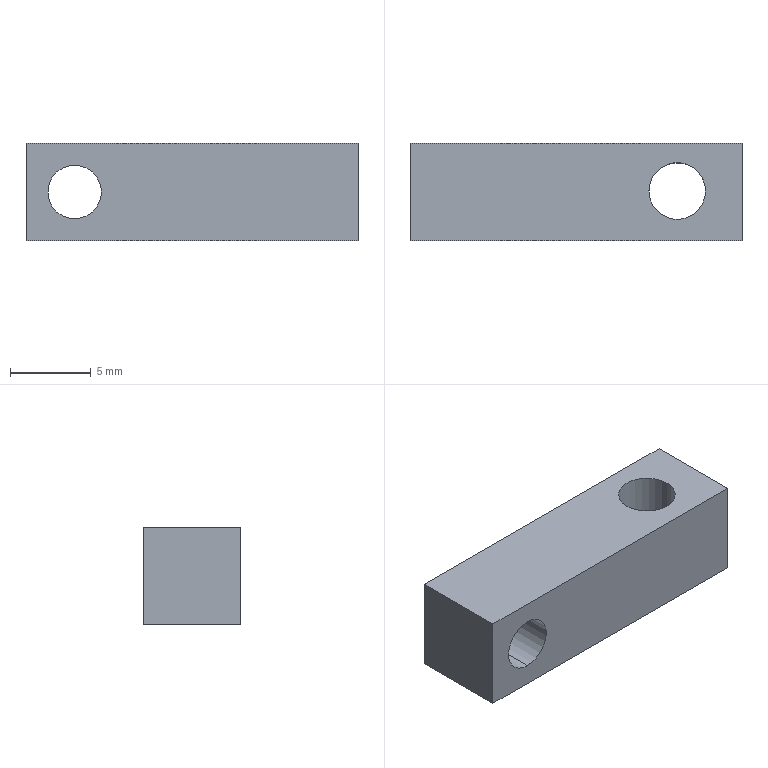Part | STEP file | Optical fiber mount | 1 solid | 10 faces | box 20.5 x 6 x 6 mm | volume 628.955 mm3 | plane 6 | cylinder 4 | commonest cylinder face diameters 3.3 x2 3.5 x2
STEP:
#1=CARTESIAN_POINT('',(0.,0.,0.));
#2=DIRECTION('',(0.,0.,1.));
#3=DIRECTION('',(1.,0.,0.));
#4=AXIS2_PLACEMENT_3D('',#1,#2,#3);
#5=CARTESIAN_POINT('',(3.,6.,1.35));
#6=VERTEX_POINT('',#5);
#7=CARTESIAN_POINT('',(3.,0.,1.35));
#8=VERTEX_POINT('',#7);
#9=CARTESIAN_POINT('',(3.,0.,1.35));
#10=DIRECTION('',(0.,-1.,0.));
#11=VECTOR('',#10,1.);
#12=LINE('',#9,#11);
#13=CARTESIAN_POINT('',(3.,0.,3.));
#14=DIRECTION('',(0.,-1.,0.));
#15=DIRECTION('',(0.,0.,-1.));
#16=AXIS2_PLACEMENT_3D('',#13,#14,#15);
#17=CYLINDRICAL_SURFACE('',#16,1.65);
#18=CARTESIAN_POINT('',(6.283,0.));
#19=DIRECTION('',(0.,1.));
#20=VECTOR('',#19,1.);
#21=LINE('',#18,#20);
#22=(GEOMETRIC_REPRESENTATION_CONTEXT(2)PARAMETRIC_REPRESENTATION_CONTEXT()REPRESENTATION_CONTEXT('',''));
#23=DEFINITIONAL_REPRESENTATION('',(#21),#22);
#24=PCURVE('',#17,#23);
#25=CARTESIAN_POINT('',(3.,0.,3.));
#26=DIRECTION('',(0.,-1.,0.));
#27=DIRECTION('',(0.,0.,-1.));
#28=AXIS2_PLACEMENT_3D('',#25,#26,#27);
#29=CYLINDRICAL_SURFACE('',#28,1.65);
#30=CARTESIAN_POINT('',(0.,0.));
#31=DIRECTION('',(0.,1.));
#32=VECTOR('',#31,1.);
#33=LINE('',#30,#32);
#34=(GEOMETRIC_REPRESENTATION_CONTEXT(2)PARAMETRIC_REPRESENTATION_CONTEXT()REPRESENTATION_CONTEXT('',''));
#35=DEFINITIONAL_REPRESENTATION('',(#33),#34);
#36=PCURVE('',#29,#35);
#37=SURFACE_CURVE('',#12,(#24,#36),.PCURVE_S1.);
#38=EDGE_CURVE('',#6,#8,#37,.T.);
#39=ORIENTED_EDGE('',*,*,#38,.T.);
#40=CARTESIAN_POINT('',(3.,0.,4.65));
#41=VERTEX_POINT('',#40);
#42=CARTESIAN_POINT('',(3.,0.,3.));
#43=DIRECTION('',(0.,-1.,0.));
#44=DIRECTION('',(0.,0.,-1.));
#45=AXIS2_PLACEMENT_3D('',#42,#43,#44);
#46=CIRCLE('',#45,1.65);
#47=CARTESIAN_POINT('',(0.,0.));
#48=DIRECTION('',(1.,0.));
#49=VECTOR('',#48,1.);
#50=LINE('',#47,#49);
#51=(GEOMETRIC_REPRESENTATION_CONTEXT(2)PARAMETRIC_REPRESENTATION_CONTEXT()REPRESENTATION_CONTEXT('',''));
#52=DEFINITIONAL_REPRESENTATION('',(#50),#51);
#53=PCURVE('',#17,#52);
#54=CARTESIAN_POINT('',(0.,0.,6.));
#55=DIRECTION('',(0.,1.,0.));
#56=DIRECTION('',(0.,0.,1.));
#57=AXIS2_PLACEMENT_3D('',#54,#55,#56);
#58=PLANE('',#57);
#59=CARTESIAN_POINT('',(-4.65,3.));
#60=CARTESIAN_POINT('',(-4.65,5.858));
#61=CARTESIAN_POINT('',(-2.175,4.429));
#62=CARTESIAN_POINT('',(0.3,3.));
#63=CARTESIAN_POINT('',(-2.175,1.571));
#64=CARTESIAN_POINT('',(-4.65,0.1421));
#65=CARTESIAN_POINT('',(-4.65,3.));
#66=(BOUNDED_CURVE()B_SPLINE_CURVE(2,(#59,#60,#61,#62,#63,#64,#65),.UNSPECIFIED.,.T.,.F.)B_SPLINE_CURVE_WITH_KNOTS((1,2,2,2,2,1),(-2.094,0.,2.094,4.189,6.283,8.378),.UNSPECIFIED.)CURVE()GEOMETRIC_REPRESENTATION_ITEM()RATIONAL_B_SPLINE_CURVE((1.,0.5,1.,0.5,1.,0.5,1.))REPRESENTATION_ITEM(''));
#67=(GEOMETRIC_REPRESENTATION_CONTEXT(2)PARAMETRIC_REPRESENTATION_CONTEXT()REPRESENTATION_CONTEXT('',''));
#68=DEFINITIONAL_REPRESENTATION('',(#66),#67);
#69=PCURVE('',#58,#68);
#70=SURFACE_CURVE('',#46,(#53,#69),.PCURVE_S1.);
#71=EDGE_CURVE('',#41,#8,#70,.T.);
#72=ORIENTED_EDGE('',*,*,#71,.F.);
#73=CARTESIAN_POINT('',(3.,6.,4.65));
#74=VERTEX_POINT('',#73);
#75=CARTESIAN_POINT('',(3.,0.,4.65));
#76=DIRECTION('',(0.,-1.,0.));
#77=VECTOR('',#76,1.);
#78=LINE('',#75,#77);
#79=CARTESIAN_POINT('',(3.142,0.));
#80=DIRECTION('',(0.,1.));
#81=VECTOR('',#80,1.);
#82=LINE('',#79,#81);
#83=(GEOMETRIC_REPRESENTATION_CONTEXT(2)PARAMETRIC_REPRESENTATION_CONTEXT()REPRESENTATION_CONTEXT('',''));
#84=DEFINITIONAL_REPRESENTATION('',(#82),#83);
#85=PCURVE('',#17,#84);
#86=CARTESIAN_POINT('',(3.142,0.));
#87=DIRECTION('',(0.,1.));
#88=VECTOR('',#87,1.);
#89=LINE('',#86,#88);
#90=(GEOMETRIC_REPRESENTATION_CONTEXT(2)PARAMETRIC_REPRESENTATION_CONTEXT()REPRESENTATION_CONTEXT('',''));
#91=DEFINITIONAL_REPRESENTATION('',(#89),#90);
#92=PCURVE('',#29,#91);
#93=SURFACE_CURVE('',#78,(#85,#92),.PCURVE_S1.);
#94=EDGE_CURVE('',#74,#41,#93,.T.);
#95=ORIENTED_EDGE('',*,*,#94,.F.);
#96=CARTESIAN_POINT('',(3.,6.,3.));
#97=DIRECTION('',(0.,-1.,0.));
#98=DIRECTION('',(0.,0.,-1.));
#99=AXIS2_PLACEMENT_3D('',#96,#97,#98);
#100=CIRCLE('',#99,1.65);
#101=CARTESIAN_POINT('',(0.,-6.));
#102=DIRECTION('',(1.,0.));
#103=VECTOR('',#102,1.);
#104=LINE('',#101,#103);
#105=(GEOMETRIC_REPRESENTATION_CONTEXT(2)PARAMETRIC_REPRESENTATION_CONTEXT()REPRESENTATION_CONTEXT('',''));
#106=DEFINITIONAL_REPRESENTATION('',(#104),#105);
#107=PCURVE('',#17,#106);
#108=CARTESIAN_POINT('',(0.,6.,6.));
#109=DIRECTION('',(0.,-1.,0.));
#110=DIRECTION('',(0.,0.,-1.));
#111=AXIS2_PLACEMENT_3D('',#108,#109,#110);
#112=PLANE('',#111);
#113=CARTESIAN_POINT('',(3.,3.));
#114=DIRECTION('',(1.,0.));
#115=AXIS2_PLACEMENT_2D('',#113,#114);
#116=CIRCLE('',#115,1.65);
#117=(GEOMETRIC_REPRESENTATION_CONTEXT(2)PARAMETRIC_REPRESENTATION_CONTEXT()REPRESENTATION_CONTEXT('',''));
#118=DEFINITIONAL_REPRESENTATION('',(#116),#117);
#119=PCURVE('',#112,#118);
#120=SURFACE_CURVE('',#100,(#107,#119),.PCURVE_S1.);
#121=EDGE_CURVE('',#74,#6,#120,.T.);
#122=ORIENTED_EDGE('',*,*,#121,.T.);
#123=EDGE_LOOP('',(#39,#72,#95,#122));
#124=FACE_BOUND('',#123,.F.);
#125=ADVANCED_FACE('',(#124),#17,.F.);
#126=CARTESIAN_POINT('',(18.25,3.058,0.));
#127=VERTEX_POINT('',#126);
#128=CARTESIAN_POINT('',(18.25,3.058,6.));
#129=VERTEX_POINT('',#128);
#130=CARTESIAN_POINT('',(18.25,3.058,0.));
#131=DIRECTION('',(0.,0.,1.));
#132=VECTOR('',#131,1.);
#133=LINE('',#130,#132);
#134=CARTESIAN_POINT('',(16.5,3.058,0.));
#135=DIRECTION('',(0.,0.,1.));
#136=DIRECTION('',(1.,0.,0.));
#137=AXIS2_PLACEMENT_3D('',#134,#135,#136);
#138=CYLINDRICAL_SURFACE('',#137,1.75);
#139=CARTESIAN_POINT('',(6.283,0.));
#140=DIRECTION('',(0.,1.));
#141=VECTOR('',#140,1.);
#142=LINE('',#139,#141);
#143=(GEOMETRIC_REPRESENTATION_CONTEXT(2)PARAMETRIC_REPRESENTATION_CONTEXT()REPRESENTATION_CONTEXT('',''));
#144=DEFINITIONAL_REPRESENTATION('',(#142),#143);
#145=PCURVE('',#138,#144);
#146=CARTESIAN_POINT('',(16.5,3.058,0.));
#147=DIRECTION('',(0.,0.,1.));
#148=DIRECTION('',(1.,0.,0.));
#149=AXIS2_PLACEMENT_3D('',#146,#147,#148);
#150=CYLINDRICAL_SURFACE('',#149,1.75);
#151=CARTESIAN_POINT('',(0.,0.));
#152=DIRECTION('',(0.,1.));
#153=VECTOR('',#152,1.);
#154=LINE('',#151,#153);
#155=(GEOMETRIC_REPRESENTATION_CONTEXT(2)PARAMETRIC_REPRESENTATION_CONTEXT()REPRESENTATION_CONTEXT('',''));
#156=DEFINITIONAL_REPRESENTATION('',(#154),#155);
#157=PCURVE('',#150,#156);
#158=SURFACE_CURVE('',#133,(#145,#157),.PCURVE_S1.);
#159=EDGE_CURVE('',#127,#129,#158,.T.);
#160=ORIENTED_EDGE('',*,*,#159,.T.);
#161=CARTESIAN_POINT('',(14.75,3.058,6.));
#162=VERTEX_POINT('',#161);
#163=CARTESIAN_POINT('',(16.5,3.058,6.));
#164=DIRECTION('',(0.,0.,1.));
#165=DIRECTION('',(1.,0.,0.));
#166=AXIS2_PLACEMENT_3D('',#163,#164,#165);
#167=CIRCLE('',#166,1.75);
#168=CARTESIAN_POINT('',(0.,6.));
#169=DIRECTION('',(1.,0.));
#170=VECTOR('',#169,1.);
#171=LINE('',#168,#170);
#172=(GEOMETRIC_REPRESENTATION_CONTEXT(2)PARAMETRIC_REPRESENTATION_CONTEXT()REPRESENTATION_CONTEXT('',''));
#173=DEFINITIONAL_REPRESENTATION('',(#171),#172);
#174=PCURVE('',#138,#173);
#175=CARTESIAN_POINT('',(0.,6.,6.));
#176=DIRECTION('',(0.,0.,-1.));
#177=DIRECTION('',(-1.,0.,0.));
#178=AXIS2_PLACEMENT_3D('',#175,#176,#177);
#179=PLANE('',#178);
#180=CARTESIAN_POINT('',(-18.25,-2.942));
#181=CARTESIAN_POINT('',(-18.25,0.08864));
#182=CARTESIAN_POINT('',(-15.625,-1.427));
#183=CARTESIAN_POINT('',(-13.,-2.942));
#184=CARTESIAN_POINT('',(-15.625,-4.458));
#185=CARTESIAN_POINT('',(-18.25,-5.974));
#186=CARTESIAN_POINT('',(-18.25,-2.942));
#187=(BOUNDED_CURVE()B_SPLINE_CURVE(2,(#180,#181,#182,#183,#184,#185,#186),.UNSPECIFIED.,.T.,.F.)B_SPLINE_CURVE_WITH_KNOTS((1,2,2,2,2,1),(-2.094,0.,2.094,4.189,6.283,8.378),.UNSPECIFIED.)CURVE()GEOMETRIC_REPRESENTATION_ITEM()RATIONAL_B_SPLINE_CURVE((1.,0.5,1.,0.5,1.,0.5,1.))REPRESENTATION_ITEM(''));
#188=(GEOMETRIC_REPRESENTATION_CONTEXT(2)PARAMETRIC_REPRESENTATION_CONTEXT()REPRESENTATION_CONTEXT('',''));
#189=DEFINITIONAL_REPRESENTATION('',(#187),#188);
#190=PCURVE('',#179,#189);
#191=SURFACE_CURVE('',#167,(#174,#190),.PCURVE_S1.);
#192=EDGE_CURVE('',#162,#129,#191,.T.);
#193=ORIENTED_EDGE('',*,*,#192,.F.);
#194=CARTESIAN_POINT('',(14.75,3.058,0.));
#195=VERTEX_POINT('',#194);
#196=CARTESIAN_POINT('',(14.75,3.058,0.));
#197=DIRECTION('',(0.,0.,1.));
#198=VECTOR('',#197,1.);
#199=LINE('',#196,#198);
#200=CARTESIAN_POINT('',(3.142,0.));
#201=DIRECTION('',(0.,1.));
#202=VECTOR('',#201,1.);
#203=LINE('',#200,#202);
#204=(GEOMETRIC_REPRESENTATION_CONTEXT(2)PARAMETRIC_REPRESENTATION_CONTEXT()REPRESENTATION_CONTEXT('',''));
#205=DEFINITIONAL_REPRESENTATION('',(#203),#204);
#206=PCURVE('',#138,#205);
#207=CARTESIAN_POINT('',(3.142,0.));
#208=DIRECTION('',(0.,1.));
#209=VECTOR('',#208,1.);
#210=LINE('',#207,#209);
#211=(GEOMETRIC_REPRESENTATION_CONTEXT(2)PARAMETRIC_REPRESENTATION_CONTEXT()REPRESENTATION_CONTEXT('',''));
#212=DEFINITIONAL_REPRESENTATION('',(#210),#211);
#213=PCURVE('',#150,#212);
#214=SURFACE_CURVE('',#199,(#206,#213),.PCURVE_S1.);
#215=EDGE_CURVE('',#195,#162,#214,.T.);
#216=ORIENTED_EDGE('',*,*,#215,.F.);
#217=CARTESIAN_POINT('',(16.5,3.058,0.));
#218=DIRECTION('',(0.,0.,1.));
#219=DIRECTION('',(1.,0.,0.));
#220=AXIS2_PLACEMENT_3D('',#217,#218,#219);
#221=CIRCLE('',#220,1.75);
#222=CARTESIAN_POINT('',(0.,0.));
#223=DIRECTION('',(1.,0.));
#224=VECTOR('',#223,1.);
#225=LINE('',#222,#224);
#226=(GEOMETRIC_REPRESENTATION_CONTEXT(2)PARAMETRIC_REPRESENTATION_CONTEXT()REPRESENTATION_CONTEXT('',''));
#227=DEFINITIONAL_REPRESENTATION('',(#225),#226);
#228=PCURVE('',#138,#227);
#229=CARTESIAN_POINT('',(0.,6.,0.));
#230=DIRECTION('',(0.,0.,-1.));
#231=DIRECTION('',(-1.,0.,0.));
#232=AXIS2_PLACEMENT_3D('',#229,#230,#231);
#233=PLANE('',#232);
#234=CARTESIAN_POINT('',(-18.25,-2.942));
#235=CARTESIAN_POINT('',(-18.25,0.08864));
#236=CARTESIAN_POINT('',(-15.625,-1.427));
#237=CARTESIAN_POINT('',(-13.,-2.942));
#238=CARTESIAN_POINT('',(-15.625,-4.458));
#239=CARTESIAN_POINT('',(-18.25,-5.974));
#240=CARTESIAN_POINT('',(-18.25,-2.942));
#241=(BOUNDED_CURVE()B_SPLINE_CURVE(2,(#234,#235,#236,#237,#238,#239,#240),.UNSPECIFIED.,.T.,.F.)B_SPLINE_CURVE_WITH_KNOTS((1,2,2,2,2,1),(-2.094,0.,2.094,4.189,6.283,8.378),.UNSPECIFIED.)CURVE()GEOMETRIC_REPRESENTATION_ITEM()RATIONAL_B_SPLINE_CURVE((1.,0.5,1.,0.5,1.,0.5,1.))REPRESENTATION_ITEM(''));
#242=(GEOMETRIC_REPRESENTATION_CONTEXT(2)PARAMETRIC_REPRESENTATION_CONTEXT()REPRESENTATION_CONTEXT('',''));
#243=DEFINITIONAL_REPRESENTATION('',(#241),#242);
#244=PCURVE('',#233,#243);
#245=SURFACE_CURVE('',#221,(#228,#244),.PCURVE_S1.);
#246=EDGE_CURVE('',#195,#127,#245,.T.);
#247=ORIENTED_EDGE('',*,*,#246,.T.);
#248=EDGE_LOOP('',(#160,#193,#216,#247));
#249=FACE_BOUND('',#248,.F.);
#250=ADVANCED_FACE('',(#249),#138,.F.);
#251=CARTESIAN_POINT('',(0.,6.,0.));
#252=VERTEX_POINT('',#251);
#253=CARTESIAN_POINT('',(0.,0.,0.));
#254=VERTEX_POINT('',#253);
#255=CARTESIAN_POINT('',(0.,0.,0.));
#256=DIRECTION('',(0.,-1.,0.));
#257=VECTOR('',#256,1.);
#258=LINE('',#255,#257);
#259=CARTESIAN_POINT('',(0.,0.,6.));
#260=DIRECTION('',(1.,0.,0.));
#261=DIRECTION('',(0.,0.,-1.));
#262=AXIS2_PLACEMENT_3D('',#259,#260,#261);
#263=PLANE('',#262);
#264=CARTESIAN_POINT('',(6.,0.));
#265=DIRECTION('',(0.,-1.));
#266=VECTOR('',#265,1.);
#267=LINE('',#264,#266);
#268=(GEOMETRIC_REPRESENTATION_CONTEXT(2)PARAMETRIC_REPRESENTATION_CONTEXT()REPRESENTATION_CONTEXT('',''));
#269=DEFINITIONAL_REPRESENTATION('',(#267),#268);
#270=PCURVE('',#263,#269);
#271=CARTESIAN_POINT('',(0.,-6.));
#272=DIRECTION('',(0.,-1.));
#273=VECTOR('',#272,1.);
#274=LINE('',#271,#273);
#275=(GEOMETRIC_REPRESENTATION_CONTEXT(2)PARAMETRIC_REPRESENTATION_CONTEXT()REPRESENTATION_CONTEXT('',''));
#276=DEFINITIONAL_REPRESENTATION('',(#274),#275);
#277=PCURVE('',#233,#276);
#278=SURFACE_CURVE('',#258,(#270,#277),.PCURVE_S1.);
#279=EDGE_CURVE('',#252,#254,#278,.T.);
#280=ORIENTED_EDGE('',*,*,#279,.T.);
#281=CARTESIAN_POINT('',(0.,0.,6.));
#282=VERTEX_POINT('',#281);
#283=CARTESIAN_POINT('',(0.,0.,6.));
#284=DIRECTION('',(0.,0.,-1.));
#285=VECTOR('',#284,1.);
#286=LINE('',#283,#285);
#287=CARTESIAN_POINT('',(0.,0.));
#288=DIRECTION('',(1.,0.));
#289=VECTOR('',#288,1.);
#290=LINE('',#287,#289);
#291=(GEOMETRIC_REPRESENTATION_CONTEXT(2)PARAMETRIC_REPRESENTATION_CONTEXT()REPRESENTATION_CONTEXT('',''));
#292=DEFINITIONAL_REPRESENTATION('',(#290),#291);
#293=PCURVE('',#263,#292);
#294=CARTESIAN_POINT('',(0.,0.));
#295=DIRECTION('',(-1.,0.));
#296=VECTOR('',#295,1.);
#297=LINE('',#294,#296);
#298=(GEOMETRIC_REPRESENTATION_CONTEXT(2)PARAMETRIC_REPRESENTATION_CONTEXT()REPRESENTATION_CONTEXT('',''));
#299=DEFINITIONAL_REPRESENTATION('',(#297),#298);
#300=PCURVE('',#58,#299);
#301=SURFACE_CURVE('',#286,(#293,#300),.PCURVE_S1.);
#302=EDGE_CURVE('',#282,#254,#301,.T.);
#303=ORIENTED_EDGE('',*,*,#302,.F.);
#304=CARTESIAN_POINT('',(0.,6.,6.));
#305=VERTEX_POINT('',#304);
#306=CARTESIAN_POINT('',(0.,0.,6.));
#307=DIRECTION('',(0.,-1.,0.));
#308=VECTOR('',#307,1.);
#309=LINE('',#306,#308);
#310=CARTESIAN_POINT('',(0.,0.));
#311=DIRECTION('',(0.,-1.));
#312=VECTOR('',#311,1.);
#313=LINE('',#310,#312);
#314=(GEOMETRIC_REPRESENTATION_CONTEXT(2)PARAMETRIC_REPRESENTATION_CONTEXT()REPRESENTATION_CONTEXT('',''));
#315=DEFINITIONAL_REPRESENTATION('',(#313),#314);
#316=PCURVE('',#263,#315);
#317=CARTESIAN_POINT('',(0.,-6.));
#318=DIRECTION('',(0.,-1.));
#319=VECTOR('',#318,1.);
#320=LINE('',#317,#319);
#321=(GEOMETRIC_REPRESENTATION_CONTEXT(2)PARAMETRIC_REPRESENTATION_CONTEXT()REPRESENTATION_CONTEXT('',''));
#322=DEFINITIONAL_REPRESENTATION('',(#320),#321);
#323=PCURVE('',#179,#322);
#324=SURFACE_CURVE('',#309,(#316,#323),.PCURVE_S1.);
#325=EDGE_CURVE('',#305,#282,#324,.T.);
#326=ORIENTED_EDGE('',*,*,#325,.F.);
#327=CARTESIAN_POINT('',(0.,6.,6.));
#328=DIRECTION('',(0.,0.,-1.));
#329=VECTOR('',#328,1.);
#330=LINE('',#327,#329);
#331=CARTESIAN_POINT('',(0.,6.));
#332=DIRECTION('',(1.,0.));
#333=VECTOR('',#332,1.);
#334=LINE('',#331,#333);
#335=(GEOMETRIC_REPRESENTATION_CONTEXT(2)PARAMETRIC_REPRESENTATION_CONTEXT()REPRESENTATION_CONTEXT('',''));
#336=DEFINITIONAL_REPRESENTATION('',(#334),#335);
#337=PCURVE('',#263,#336);
#338=CARTESIAN_POINT('',(0.,0.));
#339=DIRECTION('',(1.,0.));
#340=VECTOR('',#339,1.);
#341=LINE('',#338,#340);
#342=(GEOMETRIC_REPRESENTATION_CONTEXT(2)PARAMETRIC_REPRESENTATION_CONTEXT()REPRESENTATION_CONTEXT('',''));
#343=DEFINITIONAL_REPRESENTATION('',(#341),#342);
#344=PCURVE('',#112,#343);
#345=SURFACE_CURVE('',#330,(#337,#344),.PCURVE_S1.);
#346=EDGE_CURVE('',#305,#252,#345,.T.);
#347=ORIENTED_EDGE('',*,*,#346,.T.);
#348=EDGE_LOOP('',(#280,#303,#326,#347));
#349=FACE_BOUND('',#348,.T.);
#350=ADVANCED_FACE('',(#349),#263,.F.);
#351=CARTESIAN_POINT('',(3.,0.,3.));
#352=DIRECTION('',(0.,-1.,0.));
#353=DIRECTION('',(0.,0.,-1.));
#354=AXIS2_PLACEMENT_3D('',#351,#352,#353);
#355=CIRCLE('',#354,1.65);
#356=CARTESIAN_POINT('',(-4.65,3.));
#357=CARTESIAN_POINT('',(-4.65,5.858));
#358=CARTESIAN_POINT('',(-2.175,4.429));
#359=CARTESIAN_POINT('',(0.3,3.));
#360=CARTESIAN_POINT('',(-2.175,1.571));
#361=CARTESIAN_POINT('',(-4.65,0.1421));
#362=CARTESIAN_POINT('',(-4.65,3.));
#363=(BOUNDED_CURVE()B_SPLINE_CURVE(2,(#356,#357,#358,#359,#360,#361,#362),.UNSPECIFIED.,.T.,.F.)B_SPLINE_CURVE_WITH_KNOTS((1,2,2,2,2,1),(-2.094,0.,2.094,4.189,6.283,8.378),.UNSPECIFIED.)CURVE()GEOMETRIC_REPRESENTATION_ITEM()RATIONAL_B_SPLINE_CURVE((1.,0.5,1.,0.5,1.,0.5,1.))REPRESENTATION_ITEM(''));
#364=(GEOMETRIC_REPRESENTATION_CONTEXT(2)PARAMETRIC_REPRESENTATION_CONTEXT()REPRESENTATION_CONTEXT('',''));
#365=DEFINITIONAL_REPRESENTATION('',(#363),#364);
#366=PCURVE('',#58,#365);
#367=CARTESIAN_POINT('',(0.,0.));
#368=DIRECTION('',(1.,0.));
#369=VECTOR('',#368,1.);
#370=LINE('',#367,#369);
#371=(GEOMETRIC_REPRESENTATION_CONTEXT(2)PARAMETRIC_REPRESENTATION_CONTEXT()REPRESENTATION_CONTEXT('',''));
#372=DEFINITIONAL_REPRESENTATION('',(#370),#371);
#373=PCURVE('',#29,#372);
#374=SURFACE_CURVE('',#355,(#366,#373),.PCURVE_S1.);
#375=EDGE_CURVE('',#8,#41,#374,.T.);
#376=ORIENTED_EDGE('',*,*,#375,.F.);
#377=ORIENTED_EDGE('',*,*,#71,.F.);
#378=EDGE_LOOP('',(#376,#377));
#379=FACE_BOUND('',#378,.T.);
#380=CARTESIAN_POINT('',(20.5,0.,0.));
#381=VERTEX_POINT('',#380);
#382=CARTESIAN_POINT('',(0.,0.,0.));
#383=DIRECTION('',(1.,0.,0.));
#384=VECTOR('',#383,1.);
#385=LINE('',#382,#384);
#386=CARTESIAN_POINT('',(-6.,0.));
#387=DIRECTION('',(0.,1.));
#388=VECTOR('',#387,1.);
#389=LINE('',#386,#388);
#390=(GEOMETRIC_REPRESENTATION_CONTEXT(2)PARAMETRIC_REPRESENTATION_CONTEXT()REPRESENTATION_CONTEXT('',''));
#391=DEFINITIONAL_REPRESENTATION('',(#389),#390);
#392=PCURVE('',#58,#391);
#393=CARTESIAN_POINT('',(0.,-6.));
#394=DIRECTION('',(-1.,0.));
#395=VECTOR('',#394,1.);
#396=LINE('',#393,#395);
#397=(GEOMETRIC_REPRESENTATION_CONTEXT(2)PARAMETRIC_REPRESENTATION_CONTEXT()REPRESENTATION_CONTEXT('',''));
#398=DEFINITIONAL_REPRESENTATION('',(#396),#397);
#399=PCURVE('',#233,#398);
#400=SURFACE_CURVE('',#385,(#392,#399),.PCURVE_S1.);
#401=EDGE_CURVE('',#254,#381,#400,.T.);
#402=ORIENTED_EDGE('',*,*,#401,.T.);
#403=CARTESIAN_POINT('',(20.5,0.,6.));
#404=VERTEX_POINT('',#403);
#405=CARTESIAN_POINT('',(20.5,0.,6.));
#406=DIRECTION('',(0.,0.,-1.));
#407=VECTOR('',#406,1.);
#408=LINE('',#405,#407);
#409=CARTESIAN_POINT('',(0.,20.5));
#410=DIRECTION('',(-1.,0.));
#411=VECTOR('',#410,1.);
#412=LINE('',#409,#411);
#413=(GEOMETRIC_REPRESENTATION_CONTEXT(2)PARAMETRIC_REPRESENTATION_CONTEXT()REPRESENTATION_CONTEXT('',''));
#414=DEFINITIONAL_REPRESENTATION('',(#412),#413);
#415=PCURVE('',#58,#414);
#416=CARTESIAN_POINT('',(20.5,0.,6.));
#417=DIRECTION('',(-1.,0.,0.));
#418=DIRECTION('',(0.,0.,1.));
#419=AXIS2_PLACEMENT_3D('',#416,#417,#418);
#420=PLANE('',#419);
#421=CARTESIAN_POINT('',(0.,0.));
#422=DIRECTION('',(-1.,0.));
#423=VECTOR('',#422,1.);
#424=LINE('',#421,#423);
#425=(GEOMETRIC_REPRESENTATION_CONTEXT(2)PARAMETRIC_REPRESENTATION_CONTEXT()REPRESENTATION_CONTEXT('',''));
#426=DEFINITIONAL_REPRESENTATION('',(#424),#425);
#427=PCURVE('',#420,#426);
#428=SURFACE_CURVE('',#408,(#415,#427),.PCURVE_S1.);
#429=EDGE_CURVE('',#404,#381,#428,.T.);
#430=ORIENTED_EDGE('',*,*,#429,.F.);
#431=CARTESIAN_POINT('',(0.,0.,6.));
#432=DIRECTION('',(1.,0.,0.));
#433=VECTOR('',#432,1.);
#434=LINE('',#431,#433);
#435=CARTESIAN_POINT('',(0.,0.));
#436=DIRECTION('',(0.,1.));
#437=VECTOR('',#436,1.);
#438=LINE('',#435,#437);
#439=(GEOMETRIC_REPRESENTATION_CONTEXT(2)PARAMETRIC_REPRESENTATION_CONTEXT()REPRESENTATION_CONTEXT('',''));
#440=DEFINITIONAL_REPRESENTATION('',(#438),#439);
#441=PCURVE('',#58,#440);
#442=CARTESIAN_POINT('',(0.,-6.));
#443=DIRECTION('',(-1.,0.));
#444=VECTOR('',#443,1.);
#445=LINE('',#442,#444);
#446=(GEOMETRIC_REPRESENTATION_CONTEXT(2)PARAMETRIC_REPRESENTATION_CONTEXT()REPRESENTATION_CONTEXT('',''));
#447=DEFINITIONAL_REPRESENTATION('',(#445),#446);
#448=PCURVE('',#179,#447);
#449=SURFACE_CURVE('',#434,(#441,#448),.PCURVE_S1.);
#450=EDGE_CURVE('',#282,#404,#449,.T.);
#451=ORIENTED_EDGE('',*,*,#450,.F.);
#452=ORIENTED_EDGE('',*,*,#302,.T.);
#453=EDGE_LOOP('',(#402,#430,#451,#452));
#454=FACE_BOUND('',#453,.T.);
#455=ADVANCED_FACE('',(#379,#454),#58,.F.);
#456=CARTESIAN_POINT('',(20.5,6.,0.));
#457=VERTEX_POINT('',#456);
#458=CARTESIAN_POINT('',(20.5,0.,0.));
#459=DIRECTION('',(0.,1.,0.));
#460=VECTOR('',#459,1.);
#461=LINE('',#458,#460);
#462=CARTESIAN_POINT('',(-6.,0.));
#463=DIRECTION('',(0.,1.));
#464=VECTOR('',#463,1.);
#465=LINE('',#462,#464);
#466=(GEOMETRIC_REPRESENTATION_CONTEXT(2)PARAMETRIC_REPRESENTATION_CONTEXT()REPRESENTATION_CONTEXT('',''));
#467=DEFINITIONAL_REPRESENTATION('',(#465),#466);
#468=PCURVE('',#420,#467);
#469=CARTESIAN_POINT('',(-20.5,-6.));
#470=DIRECTION('',(0.,1.));
#471=VECTOR('',#470,1.);
#472=LINE('',#469,#471);
#473=(GEOMETRIC_REPRESENTATION_CONTEXT(2)PARAMETRIC_REPRESENTATION_CONTEXT()REPRESENTATION_CONTEXT('',''));
#474=DEFINITIONAL_REPRESENTATION('',(#472),#473);
#475=PCURVE('',#233,#474);
#476=SURFACE_CURVE('',#461,(#468,#475),.PCURVE_S1.);
#477=EDGE_CURVE('',#381,#457,#476,.T.);
#478=ORIENTED_EDGE('',*,*,#477,.T.);
#479=CARTESIAN_POINT('',(20.5,6.,6.));
#480=VERTEX_POINT('',#479);
#481=CARTESIAN_POINT('',(20.5,6.,6.));
#482=DIRECTION('',(0.,0.,-1.));
#483=VECTOR('',#482,1.);
#484=LINE('',#481,#483);
#485=CARTESIAN_POINT('',(0.,6.));
#486=DIRECTION('',(-1.,0.));
#487=VECTOR('',#486,1.);
#488=LINE('',#485,#487);
#489=(GEOMETRIC_REPRESENTATION_CONTEXT(2)PARAMETRIC_REPRESENTATION_CONTEXT()REPRESENTATION_CONTEXT('',''));
#490=DEFINITIONAL_REPRESENTATION('',(#488),#489);
#491=PCURVE('',#420,#490);
#492=CARTESIAN_POINT('',(0.,20.5));
#493=DIRECTION('',(1.,0.));
#494=VECTOR('',#493,1.);
#495=LINE('',#492,#494);
#496=(GEOMETRIC_REPRESENTATION_CONTEXT(2)PARAMETRIC_REPRESENTATION_CONTEXT()REPRESENTATION_CONTEXT('',''));
#497=DEFINITIONAL_REPRESENTATION('',(#495),#496);
#498=PCURVE('',#112,#497);
#499=SURFACE_CURVE('',#484,(#491,#498),.PCURVE_S1.);
#500=EDGE_CURVE('',#480,#457,#499,.T.);
#501=ORIENTED_EDGE('',*,*,#500,.F.);
#502=CARTESIAN_POINT('',(20.5,0.,6.));
#503=DIRECTION('',(0.,1.,0.));
#504=VECTOR('',#503,1.);
#505=LINE('',#502,#504);
#506=CARTESIAN_POINT('',(0.,0.));
#507=DIRECTION('',(0.,1.));
#508=VECTOR('',#507,1.);
#509=LINE('',#506,#508);
#510=(GEOMETRIC_REPRESENTATION_CONTEXT(2)PARAMETRIC_REPRESENTATION_CONTEXT()REPRESENTATION_CONTEXT('',''));
#511=DEFINITIONAL_REPRESENTATION('',(#509),#510);
#512=PCURVE('',#420,#511);
#513=CARTESIAN_POINT('',(-20.5,-6.));
#514=DIRECTION('',(0.,1.));
#515=VECTOR('',#514,1.);
#516=LINE('',#513,#515);
#517=(GEOMETRIC_REPRESENTATION_CONTEXT(2)PARAMETRIC_REPRESENTATION_CONTEXT()REPRESENTATION_CONTEXT('',''));
#518=DEFINITIONAL_REPRESENTATION('',(#516),#517);
#519=PCURVE('',#179,#518);
#520=SURFACE_CURVE('',#505,(#512,#519),.PCURVE_S1.);
#521=EDGE_CURVE('',#404,#480,#520,.T.);
#522=ORIENTED_EDGE('',*,*,#521,.F.);
#523=ORIENTED_EDGE('',*,*,#429,.T.);
#524=EDGE_LOOP('',(#478,#501,#522,#523));
#525=FACE_BOUND('',#524,.T.);
#526=ADVANCED_FACE('',(#525),#420,.F.);
#527=CARTESIAN_POINT('',(3.,6.,3.));
#528=DIRECTION('',(0.,-1.,0.));
#529=DIRECTION('',(0.,0.,-1.));
#530=AXIS2_PLACEMENT_3D('',#527,#528,#529);
#531=CIRCLE('',#530,1.65);
#532=CARTESIAN_POINT('',(3.,3.));
#533=DIRECTION('',(1.,0.));
#534=AXIS2_PLACEMENT_2D('',#532,#533);
#535=CIRCLE('',#534,1.65);
#536=(GEOMETRIC_REPRESENTATION_CONTEXT(2)PARAMETRIC_REPRESENTATION_CONTEXT()REPRESENTATION_CONTEXT('',''));
#537=DEFINITIONAL_REPRESENTATION('',(#535),#536);
#538=PCURVE('',#112,#537);
#539=CARTESIAN_POINT('',(0.,-6.));
#540=DIRECTION('',(1.,0.));
#541=VECTOR('',#540,1.);
#542=LINE('',#539,#541);
#543=(GEOMETRIC_REPRESENTATION_CONTEXT(2)PARAMETRIC_REPRESENTATION_CONTEXT()REPRESENTATION_CONTEXT('',''));
#544=DEFINITIONAL_REPRESENTATION('',(#542),#543);
#545=PCURVE('',#29,#544);
#546=SURFACE_CURVE('',#531,(#538,#545),.PCURVE_S1.);
#547=EDGE_CURVE('',#6,#74,#546,.T.);
#548=ORIENTED_EDGE('',*,*,#547,.T.);
#549=ORIENTED_EDGE('',*,*,#121,.T.);
#550=EDGE_LOOP('',(#548,#549));
#551=FACE_BOUND('',#550,.T.);
#552=CARTESIAN_POINT('',(0.,6.,0.));
#553=DIRECTION('',(-1.,0.,0.));
#554=VECTOR('',#553,1.);
#555=LINE('',#552,#554);
#556=CARTESIAN_POINT('',(6.,0.));
#557=DIRECTION('',(0.,-1.));
#558=VECTOR('',#557,1.);
#559=LINE('',#556,#558);
#560=(GEOMETRIC_REPRESENTATION_CONTEXT(2)PARAMETRIC_REPRESENTATION_CONTEXT()REPRESENTATION_CONTEXT('',''));
#561=DEFINITIONAL_REPRESENTATION('',(#559),#560);
#562=PCURVE('',#112,#561);
#563=CARTESIAN_POINT('',(0.,0.));
#564=DIRECTION('',(1.,0.));
#565=VECTOR('',#564,1.);
#566=LINE('',#563,#565);
#567=(GEOMETRIC_REPRESENTATION_CONTEXT(2)PARAMETRIC_REPRESENTATION_CONTEXT()REPRESENTATION_CONTEXT('',''));
#568=DEFINITIONAL_REPRESENTATION('',(#566),#567);
#569=PCURVE('',#233,#568);
#570=SURFACE_CURVE('',#555,(#562,#569),.PCURVE_S1.);
#571=EDGE_CURVE('',#457,#252,#570,.T.);
#572=ORIENTED_EDGE('',*,*,#571,.T.);
#573=ORIENTED_EDGE('',*,*,#346,.F.);
#574=CARTESIAN_POINT('',(0.,6.,6.));
#575=DIRECTION('',(-1.,0.,0.));
#576=VECTOR('',#575,1.);
#577=LINE('',#574,#576);
#578=CARTESIAN_POINT('',(0.,0.));
#579=DIRECTION('',(0.,-1.));
#580=VECTOR('',#579,1.);
#581=LINE('',#578,#580);
#582=(GEOMETRIC_REPRESENTATION_CONTEXT(2)PARAMETRIC_REPRESENTATION_CONTEXT()REPRESENTATION_CONTEXT('',''));
#583=DEFINITIONAL_REPRESENTATION('',(#581),#582);
#584=PCURVE('',#112,#583);
#585=CARTESIAN_POINT('',(0.,0.));
#586=DIRECTION('',(1.,0.));
#587=VECTOR('',#586,1.);
#588=LINE('',#585,#587);
#589=(GEOMETRIC_REPRESENTATION_CONTEXT(2)PARAMETRIC_REPRESENTATION_CONTEXT()REPRESENTATION_CONTEXT('',''));
#590=DEFINITIONAL_REPRESENTATION('',(#588),#589);
#591=PCURVE('',#179,#590);
#592=SURFACE_CURVE('',#577,(#584,#591),.PCURVE_S1.);
#593=EDGE_CURVE('',#480,#305,#592,.T.);
#594=ORIENTED_EDGE('',*,*,#593,.F.);
#595=ORIENTED_EDGE('',*,*,#500,.T.);
#596=EDGE_LOOP('',(#572,#573,#594,#595));
#597=FACE_BOUND('',#596,.T.);
#598=ADVANCED_FACE('',(#551,#597),#112,.F.);
#599=CARTESIAN_POINT('',(16.5,3.058,6.));
#600=DIRECTION('',(0.,0.,1.));
#601=DIRECTION('',(1.,0.,0.));
#602=AXIS2_PLACEMENT_3D('',#599,#600,#601);
#603=CIRCLE('',#602,1.75);
#604=CARTESIAN_POINT('',(-18.25,-2.942));
#605=CARTESIAN_POINT('',(-18.25,0.08864));
#606=CARTESIAN_POINT('',(-15.625,-1.427));
#607=CARTESIAN_POINT('',(-13.,-2.942));
#608=CARTESIAN_POINT('',(-15.625,-4.458));
#609=CARTESIAN_POINT('',(-18.25,-5.974));
#610=CARTESIAN_POINT('',(-18.25,-2.942));
#611=(BOUNDED_CURVE()B_SPLINE_CURVE(2,(#604,#605,#606,#607,#608,#609,#610),.UNSPECIFIED.,.T.,.F.)B_SPLINE_CURVE_WITH_KNOTS((1,2,2,2,2,1),(-2.094,0.,2.094,4.189,6.283,8.378),.UNSPECIFIED.)CURVE()GEOMETRIC_REPRESENTATION_ITEM()RATIONAL_B_SPLINE_CURVE((1.,0.5,1.,0.5,1.,0.5,1.))REPRESENTATION_ITEM(''));
#612=(GEOMETRIC_REPRESENTATION_CONTEXT(2)PARAMETRIC_REPRESENTATION_CONTEXT()REPRESENTATION_CONTEXT('',''));
#613=DEFINITIONAL_REPRESENTATION('',(#611),#612);
#614=PCURVE('',#179,#613);
#615=CARTESIAN_POINT('',(0.,6.));
#616=DIRECTION('',(1.,0.));
#617=VECTOR('',#616,1.);
#618=LINE('',#615,#617);
#619=(GEOMETRIC_REPRESENTATION_CONTEXT(2)PARAMETRIC_REPRESENTATION_CONTEXT()REPRESENTATION_CONTEXT('',''));
#620=DEFINITIONAL_REPRESENTATION('',(#618),#619);
#621=PCURVE('',#150,#620);
#622=SURFACE_CURVE('',#603,(#614,#621),.PCURVE_S1.);
#623=EDGE_CURVE('',#129,#162,#622,.T.);
#624=ORIENTED_EDGE('',*,*,#623,.F.);
#625=ORIENTED_EDGE('',*,*,#192,.F.);
#626=EDGE_LOOP('',(#624,#625));
#627=FACE_BOUND('',#626,.T.);
#628=ORIENTED_EDGE('',*,*,#325,.T.);
#629=ORIENTED_EDGE('',*,*,#450,.T.);
#630=ORIENTED_EDGE('',*,*,#521,.T.);
#631=ORIENTED_EDGE('',*,*,#593,.T.);
#632=EDGE_LOOP('',(#628,#629,#630,#631));
#633=FACE_BOUND('',#632,.T.);
#634=ADVANCED_FACE('',(#627,#633),#179,.F.);
#635=CARTESIAN_POINT('',(16.5,3.058,0.));
#636=DIRECTION('',(0.,0.,1.));
#637=DIRECTION('',(1.,0.,0.));
#638=AXIS2_PLACEMENT_3D('',#635,#636,#637);
#639=CIRCLE('',#638,1.75);
#640=CARTESIAN_POINT('',(-18.25,-2.942));
#641=CARTESIAN_POINT('',(-18.25,0.08864));
#642=CARTESIAN_POINT('',(-15.625,-1.427));
#643=CARTESIAN_POINT('',(-13.,-2.942));
#644=CARTESIAN_POINT('',(-15.625,-4.458));
#645=CARTESIAN_POINT('',(-18.25,-5.974));
#646=CARTESIAN_POINT('',(-18.25,-2.942));
#647=(BOUNDED_CURVE()B_SPLINE_CURVE(2,(#640,#641,#642,#643,#644,#645,#646),.UNSPECIFIED.,.T.,.F.)B_SPLINE_CURVE_WITH_KNOTS((1,2,2,2,2,1),(-2.094,0.,2.094,4.189,6.283,8.378),.UNSPECIFIED.)CURVE()GEOMETRIC_REPRESENTATION_ITEM()RATIONAL_B_SPLINE_CURVE((1.,0.5,1.,0.5,1.,0.5,1.))REPRESENTATION_ITEM(''));
#648=(GEOMETRIC_REPRESENTATION_CONTEXT(2)PARAMETRIC_REPRESENTATION_CONTEXT()REPRESENTATION_CONTEXT('',''));
#649=DEFINITIONAL_REPRESENTATION('',(#647),#648);
#650=PCURVE('',#233,#649);
#651=CARTESIAN_POINT('',(0.,0.));
#652=DIRECTION('',(1.,0.));
#653=VECTOR('',#652,1.);
#654=LINE('',#651,#653);
#655=(GEOMETRIC_REPRESENTATION_CONTEXT(2)PARAMETRIC_REPRESENTATION_CONTEXT()REPRESENTATION_CONTEXT('',''));
#656=DEFINITIONAL_REPRESENTATION('',(#654),#655);
#657=PCURVE('',#150,#656);
#658=SURFACE_CURVE('',#639,(#650,#657),.PCURVE_S1.);
#659=EDGE_CURVE('',#127,#195,#658,.T.);
#660=ORIENTED_EDGE('',*,*,#659,.T.);
#661=ORIENTED_EDGE('',*,*,#246,.T.);
#662=EDGE_LOOP('',(#660,#661));
#663=FACE_BOUND('',#662,.T.);
#664=ORIENTED_EDGE('',*,*,#279,.F.);
#665=ORIENTED_EDGE('',*,*,#571,.F.);
#666=ORIENTED_EDGE('',*,*,#477,.F.);
#667=ORIENTED_EDGE('',*,*,#401,.F.);
#668=EDGE_LOOP('',(#664,#665,#666,#667));
#669=FACE_BOUND('',#668,.T.);
#670=ADVANCED_FACE('',(#663,#669),#233,.T.);
#671=ORIENTED_EDGE('',*,*,#623,.F.);
#672=ORIENTED_EDGE('',*,*,#159,.F.);
#673=ORIENTED_EDGE('',*,*,#659,.T.);
#674=ORIENTED_EDGE('',*,*,#215,.T.);
#675=EDGE_LOOP('',(#671,#672,#673,#674));
#676=FACE_BOUND('',#675,.F.);
#677=ADVANCED_FACE('',(#676),#150,.F.);
#678=ORIENTED_EDGE('',*,*,#375,.F.);
#679=ORIENTED_EDGE('',*,*,#38,.F.);
#680=ORIENTED_EDGE('',*,*,#547,.T.);
#681=ORIENTED_EDGE('',*,*,#94,.T.);
#682=EDGE_LOOP('',(#678,#679,#680,#681));
#683=FACE_BOUND('',#682,.F.);
#684=ADVANCED_FACE('',(#683),#29,.F.);
#685=CLOSED_SHELL('',(#125,#250,#350,#455,#526,#598,#634,#670,#677,#684));
#686=MANIFOLD_SOLID_BREP('',#685);
#687=(LENGTH_UNIT()NAMED_UNIT(*)SI_UNIT(.MILLI.,.METRE.));
#688=UNCERTAINTY_MEASURE_WITH_UNIT(LENGTH_MEASURE(0.0000001),#687,'','');
#689=(NAMED_UNIT(*)PLANE_ANGLE_UNIT()SI_UNIT($,.RADIAN.));
#690=(NAMED_UNIT(*)SI_UNIT($,.STERADIAN.)SOLID_ANGLE_UNIT());
#691=(GEOMETRIC_REPRESENTATION_CONTEXT(3)GLOBAL_UNCERTAINTY_ASSIGNED_CONTEXT((#688))GLOBAL_UNIT_ASSIGNED_CONTEXT((#687,#689,#690))REPRESENTATION_CONTEXT('',''));
#692=ADVANCED_BREP_SHAPE_REPRESENTATION('',(#4,#686),#691);